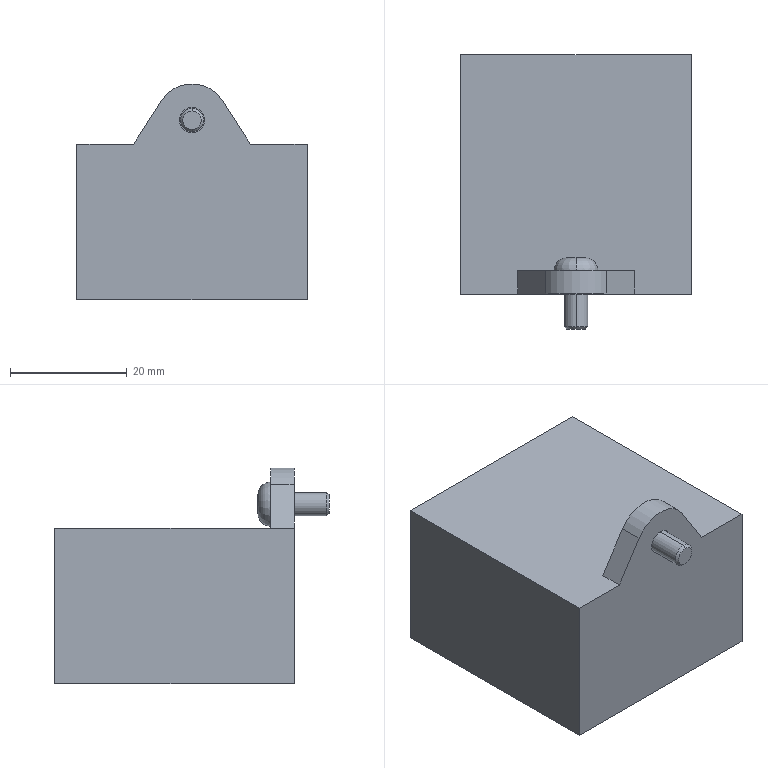Part | SolidWorks | features RefAxis 3, ICE 2, 3DProfileFeature 1, Extrusion 1, RevCut 1, Revolution 1 | 1 solid | 28 faces | box 39.5 x 47 x 37 mm | volume 43916 mm3 | plane 19 | cylinder 5 | torus 2 | cone 2 | commonest cylinder face diameters 4 x2 4.3 x2 12.4 x1
STEP:
#1=CARTESIAN_POINT('',(0.,4.,7.9));
#2=VERTEX_POINT('',#1);
#3=CARTESIAN_POINT('',(0.,4.,0.3));
#4=VERTEX_POINT('',#3);
#5=CARTESIAN_POINT('',(0.,4.,4.1));
#6=DIRECTION('',(0.,1.,0.));
#7=DIRECTION('',(0.,0.,1.));
#8=AXIS2_PLACEMENT_3D('',#5,#6,#7);
#9=CIRCLE('',#8,3.8);
#10=EDGE_CURVE('',#2,#4,#9,.T.);
#11=ORIENTED_EDGE('',*,*,#10,.T.);
#12=CARTESIAN_POINT('',(0.,6.2,2.5));
#13=VERTEX_POINT('',#12);
#14=CARTESIAN_POINT('',(0.,4.,2.5));
#15=DIRECTION('',(1.,0.,0.));
#16=DIRECTION('',(0.,0.,-1.));
#17=AXIS2_PLACEMENT_3D('',#14,#15,#16);
#18=CIRCLE('',#17,2.2);
#19=EDGE_CURVE('',#4,#13,#18,.T.);
#20=ORIENTED_EDGE('',*,*,#19,.T.);
#21=CARTESIAN_POINT('',(0.,6.2,5.7));
#22=VERTEX_POINT('',#21);
#23=CARTESIAN_POINT('',(0.,6.2,4.1));
#24=DIRECTION('',(0.,1.,0.));
#25=DIRECTION('',(0.,0.,1.));
#26=AXIS2_PLACEMENT_3D('',#23,#24,#25);
#27=CIRCLE('',#26,1.6);
#28=EDGE_CURVE('',#22,#13,#27,.T.);
#29=ORIENTED_EDGE('',*,*,#28,.F.);
#30=CARTESIAN_POINT('',(0.,4.,5.7));
#31=DIRECTION('',(-1.,0.,0.));
#32=DIRECTION('',(0.,0.,1.));
#33=AXIS2_PLACEMENT_3D('',#30,#31,#32);
#34=CIRCLE('',#33,2.2);
#35=EDGE_CURVE('',#2,#22,#34,.T.);
#36=ORIENTED_EDGE('',*,*,#35,.F.);
#37=EDGE_LOOP('',(#11,#20,#29,#36));
#38=FACE_OUTER_BOUND('',#37,.T.);
#39=CARTESIAN_POINT('',(0.,4.,4.1));
#40=DIRECTION('',(0.,1.,0.));
#41=DIRECTION('',(0.,0.,1.));
#42=AXIS2_PLACEMENT_3D('',#39,#40,#41);
#43=TOROIDAL_SURFACE('',#42,1.6,2.2);
#44=ADVANCED_FACE('',(#38),#43,.T.);
#45=CARTESIAN_POINT('',(0.,-5.57,6.1));
#46=VERTEX_POINT('',#45);
#47=CARTESIAN_POINT('',(0.,-5.57,2.1));
#48=VERTEX_POINT('',#47);
#49=CARTESIAN_POINT('',(0.,-5.57,4.1));
#50=DIRECTION('',(0.,1.,0.));
#51=DIRECTION('',(0.,0.,1.));
#52=AXIS2_PLACEMENT_3D('',#49,#50,#51);
#53=CIRCLE('',#52,2.);
#54=EDGE_CURVE('',#46,#48,#53,.T.);
#55=ORIENTED_EDGE('',*,*,#54,.T.);
#56=CARTESIAN_POINT('',(0.,4.,2.1));
#57=VERTEX_POINT('',#56);
#58=CARTESIAN_POINT('',(0.,-6.,2.1));
#59=DIRECTION('',(0.,1.,0.));
#60=VECTOR('',#59,1000.);
#61=LINE('',#58,#60);
#62=EDGE_CURVE('',#48,#57,#61,.T.);
#63=ORIENTED_EDGE('',*,*,#62,.T.);
#64=CARTESIAN_POINT('',(0.,4.,6.1));
#65=VERTEX_POINT('',#64);
#66=CARTESIAN_POINT('',(0.,4.,4.1));
#67=DIRECTION('',(0.,1.,0.));
#68=DIRECTION('',(0.,0.,1.));
#69=AXIS2_PLACEMENT_3D('',#66,#67,#68);
#70=CIRCLE('',#69,2.);
#71=EDGE_CURVE('',#65,#57,#70,.T.);
#72=ORIENTED_EDGE('',*,*,#71,.F.);
#73=CARTESIAN_POINT('',(0.,-6.,6.1));
#74=DIRECTION('',(0.,1.,0.));
#75=VECTOR('',#74,1000.);
#76=LINE('',#73,#75);
#77=EDGE_CURVE('',#46,#65,#76,.T.);
#78=ORIENTED_EDGE('',*,*,#77,.F.);
#79=EDGE_LOOP('',(#55,#63,#72,#78));
#80=FACE_OUTER_BOUND('',#79,.T.);
#81=CARTESIAN_POINT('',(0.,-6.,4.1));
#82=DIRECTION('',(0.,1.,0.));
#83=DIRECTION('',(0.,0.,1.));
#84=AXIS2_PLACEMENT_3D('',#81,#82,#83);
#85=CYLINDRICAL_SURFACE('',#84,2.);
#86=ADVANCED_FACE('',(#80),#85,.T.);
#87=CARTESIAN_POINT('',(0.,-6.,5.671));
#88=VERTEX_POINT('',#87);
#89=CARTESIAN_POINT('',(0.,-6.,2.53));
#90=VERTEX_POINT('',#89);
#91=CARTESIAN_POINT('',(0.,-6.,4.1));
#92=DIRECTION('',(0.,1.,0.));
#93=DIRECTION('',(0.,0.,1.));
#94=AXIS2_PLACEMENT_3D('',#91,#92,#93);
#95=CIRCLE('',#94,1.57);
#96=EDGE_CURVE('',#88,#90,#95,.T.);
#97=ORIENTED_EDGE('',*,*,#96,.T.);
#98=CARTESIAN_POINT('',(0.,-6.,2.53));
#99=DIRECTION('',(0.,0.7071,-0.7071));
#100=VECTOR('',#99,1000.);
#101=LINE('',#98,#100);
#102=EDGE_CURVE('',#90,#48,#101,.T.);
#103=ORIENTED_EDGE('',*,*,#102,.T.);
#104=ORIENTED_EDGE('',*,*,#54,.F.);
#105=CARTESIAN_POINT('',(0.,-6.,5.671));
#106=DIRECTION('',(0.,0.7071,0.7071));
#107=VECTOR('',#106,1000.);
#108=LINE('',#105,#107);
#109=EDGE_CURVE('',#88,#46,#108,.T.);
#110=ORIENTED_EDGE('',*,*,#109,.F.);
#111=EDGE_LOOP('',(#97,#103,#104,#110));
#112=FACE_OUTER_BOUND('',#111,.T.);
#113=CARTESIAN_POINT('',(0.,-6.,4.1));
#114=DIRECTION('',(0.,1.,0.));
#115=DIRECTION('',(0.,0.,1.));
#116=AXIS2_PLACEMENT_3D('',#113,#114,#115);
#117=CONICAL_SURFACE('',#116,1.57,0.7854);
#118=ADVANCED_FACE('',(#112),#117,.T.);
#119=CARTESIAN_POINT('',(0.,0.,1.95));
#120=VERTEX_POINT('',#119);
#121=CARTESIAN_POINT('',(0.,0.,6.25));
#122=VERTEX_POINT('',#121);
#123=CARTESIAN_POINT('',(0.,0.,4.1));
#124=DIRECTION('',(0.,1.,0.));
#125=DIRECTION('',(0.,0.,1.));
#126=AXIS2_PLACEMENT_3D('',#123,#124,#125);
#127=CIRCLE('',#126,2.15);
#128=EDGE_CURVE('',#120,#122,#127,.T.);
#129=ORIENTED_EDGE('',*,*,#128,.F.);
#130=CARTESIAN_POINT('',(0.,4.,1.95));
#131=VERTEX_POINT('',#130);
#132=CARTESIAN_POINT('',(0.,0.,1.95));
#133=DIRECTION('',(0.,1.,0.));
#134=VECTOR('',#133,1000.);
#135=LINE('',#132,#134);
#136=EDGE_CURVE('',#120,#131,#135,.T.);
#137=ORIENTED_EDGE('',*,*,#136,.T.);
#138=CARTESIAN_POINT('',(0.,4.,6.25));
#139=VERTEX_POINT('',#138);
#140=CARTESIAN_POINT('',(0.,4.,4.1));
#141=DIRECTION('',(0.,1.,0.));
#142=DIRECTION('',(0.,0.,1.));
#143=AXIS2_PLACEMENT_3D('',#140,#141,#142);
#144=CIRCLE('',#143,2.15);
#145=EDGE_CURVE('',#131,#139,#144,.T.);
#146=ORIENTED_EDGE('',*,*,#145,.T.);
#147=CARTESIAN_POINT('',(0.,0.,6.25));
#148=DIRECTION('',(0.,1.,0.));
#149=VECTOR('',#148,1000.);
#150=LINE('',#147,#149);
#151=EDGE_CURVE('',#122,#139,#150,.T.);
#152=ORIENTED_EDGE('',*,*,#151,.F.);
#153=EDGE_LOOP('',(#129,#137,#146,#152));
#154=FACE_OUTER_BOUND('',#153,.T.);
#155=CARTESIAN_POINT('',(0.,0.,4.1));
#156=DIRECTION('',(0.,1.,0.));
#157=DIRECTION('',(0.,0.,1.));
#158=AXIS2_PLACEMENT_3D('',#155,#156,#157);
#159=CYLINDRICAL_SURFACE('',#158,2.15);
#160=ADVANCED_FACE('',(#154),#159,.F.);
#161=CARTESIAN_POINT('',(10.,4.,0.));
#162=VERTEX_POINT('',#161);
#163=CARTESIAN_POINT('',(-10.,4.,0.));
#164=VERTEX_POINT('',#163);
#165=CARTESIAN_POINT('',(10.,4.,0.));
#166=DIRECTION('',(-1.,0.,0.));
#167=VECTOR('',#166,1000.);
#168=LINE('',#165,#167);
#169=EDGE_CURVE('',#162,#164,#168,.T.);
#170=ORIENTED_EDGE('',*,*,#169,.T.);
#171=CARTESIAN_POINT('',(-5.217,4.,7.45));
#172=VERTEX_POINT('',#171);
#173=CARTESIAN_POINT('',(-10.,4.,0.));
#174=DIRECTION('',(0.5403,0.,0.8415));
#175=VECTOR('',#174,1000.);
#176=LINE('',#173,#175);
#177=EDGE_CURVE('',#164,#172,#176,.T.);
#178=ORIENTED_EDGE('',*,*,#177,.T.);
#179=CARTESIAN_POINT('',(5.217,4.,7.45));
#180=VERTEX_POINT('',#179);
#181=CARTESIAN_POINT('',(0.,4.,4.1));
#182=DIRECTION('',(0.,1.,0.));
#183=DIRECTION('',(0.,0.,1.));
#184=AXIS2_PLACEMENT_3D('',#181,#182,#183);
#185=CIRCLE('',#184,6.2);
#186=EDGE_CURVE('',#172,#180,#185,.T.);
#187=ORIENTED_EDGE('',*,*,#186,.T.);
#188=CARTESIAN_POINT('',(5.217,4.,7.45));
#189=DIRECTION('',(0.5403,0.,-0.8415));
#190=VECTOR('',#189,1000.);
#191=LINE('',#188,#190);
#192=EDGE_CURVE('',#180,#162,#191,.T.);
#193=ORIENTED_EDGE('',*,*,#192,.T.);
#194=EDGE_LOOP('',(#170,#178,#187,#193));
#195=FACE_OUTER_BOUND('',#194,.T.);
#196=ORIENTED_EDGE('',*,*,#10,.F.);
#197=CARTESIAN_POINT('',(0.,4.,4.1));
#198=DIRECTION('',(0.,1.,0.));
#199=DIRECTION('',(0.,0.,1.));
#200=AXIS2_PLACEMENT_3D('',#197,#198,#199);
#201=CIRCLE('',#200,3.8);
#202=EDGE_CURVE('',#4,#2,#201,.T.);
#203=ORIENTED_EDGE('',*,*,#202,.F.);
#204=EDGE_LOOP('',(#196,#203));
#205=FACE_BOUND('',#204,.T.);
#206=CARTESIAN_POINT('',(0.,4.,4.1));
#207=DIRECTION('',(0.,1.,0.));
#208=DIRECTION('',(0.,0.,1.));
#209=AXIS2_PLACEMENT_3D('',#206,#207,#208);
#210=PLANE('',#209);
#211=ADVANCED_FACE('',(#195,#205),#210,.T.);
#212=CARTESIAN_POINT('',(-19.75,0.,-26.7));
#213=VERTEX_POINT('',#212);
#214=CARTESIAN_POINT('',(-19.75,0.,0.));
#215=VERTEX_POINT('',#214);
#216=CARTESIAN_POINT('',(-19.75,0.,-26.7));
#217=DIRECTION('',(0.,0.,1.));
#218=VECTOR('',#217,1000.);
#219=LINE('',#216,#218);
#220=EDGE_CURVE('',#213,#215,#219,.T.);
#221=ORIENTED_EDGE('',*,*,#220,.F.);
#222=CARTESIAN_POINT('',(19.75,0.,-26.7));
#223=VERTEX_POINT('',#222);
#224=CARTESIAN_POINT('',(19.75,0.,-26.7));
#225=DIRECTION('',(-1.,0.,0.));
#226=VECTOR('',#225,1000.);
#227=LINE('',#224,#226);
#228=EDGE_CURVE('',#223,#213,#227,.T.);
#229=ORIENTED_EDGE('',*,*,#228,.F.);
#230=CARTESIAN_POINT('',(19.75,0.,0.));
#231=VERTEX_POINT('',#230);
#232=CARTESIAN_POINT('',(19.75,0.,0.));
#233=DIRECTION('',(0.,0.,-1.));
#234=VECTOR('',#233,1000.);
#235=LINE('',#232,#234);
#236=EDGE_CURVE('',#231,#223,#235,.T.);
#237=ORIENTED_EDGE('',*,*,#236,.F.);
#238=CARTESIAN_POINT('',(10.,0.,0.));
#239=VERTEX_POINT('',#238);
#240=CARTESIAN_POINT('',(-19.75,0.,0.));
#241=DIRECTION('',(1.,0.,0.));
#242=VECTOR('',#241,1000.);
#243=LINE('',#240,#242);
#244=EDGE_CURVE('',#239,#231,#243,.T.);
#245=ORIENTED_EDGE('',*,*,#244,.F.);
#246=CARTESIAN_POINT('',(5.217,0.,7.45));
#247=VERTEX_POINT('',#246);
#248=CARTESIAN_POINT('',(5.217,0.,7.45));
#249=DIRECTION('',(0.5403,0.,-0.8415));
#250=VECTOR('',#249,1000.);
#251=LINE('',#248,#250);
#252=EDGE_CURVE('',#247,#239,#251,.T.);
#253=ORIENTED_EDGE('',*,*,#252,.F.);
#254=CARTESIAN_POINT('',(-5.217,0.,7.45));
#255=VERTEX_POINT('',#254);
#256=CARTESIAN_POINT('',(0.,0.,4.1));
#257=DIRECTION('',(0.,1.,0.));
#258=DIRECTION('',(0.,0.,1.));
#259=AXIS2_PLACEMENT_3D('',#256,#257,#258);
#260=CIRCLE('',#259,6.2);
#261=EDGE_CURVE('',#255,#247,#260,.T.);
#262=ORIENTED_EDGE('',*,*,#261,.F.);
#263=CARTESIAN_POINT('',(-10.,0.,0.));
#264=VERTEX_POINT('',#263);
#265=CARTESIAN_POINT('',(-10.,0.,0.));
#266=DIRECTION('',(0.5403,0.,0.8415));
#267=VECTOR('',#266,1000.);
#268=LINE('',#265,#267);
#269=EDGE_CURVE('',#264,#255,#268,.T.);
#270=ORIENTED_EDGE('',*,*,#269,.F.);
#271=CARTESIAN_POINT('',(-19.75,0.,0.));
#272=DIRECTION('',(1.,0.,0.));
#273=VECTOR('',#272,1000.);
#274=LINE('',#271,#273);
#275=EDGE_CURVE('',#215,#264,#274,.T.);
#276=ORIENTED_EDGE('',*,*,#275,.F.);
#277=EDGE_LOOP('',(#221,#229,#237,#245,#253,#262,#270,#276));
#278=FACE_OUTER_BOUND('',#277,.T.);
#279=CARTESIAN_POINT('',(0.,0.,4.1));
#280=DIRECTION('',(0.,1.,0.));
#281=DIRECTION('',(0.,0.,1.));
#282=AXIS2_PLACEMENT_3D('',#279,#280,#281);
#283=CIRCLE('',#282,2.15);
#284=EDGE_CURVE('',#122,#120,#283,.T.);
#285=ORIENTED_EDGE('',*,*,#284,.T.);
#286=ORIENTED_EDGE('',*,*,#128,.T.);
#287=EDGE_LOOP('',(#285,#286));
#288=FACE_BOUND('',#287,.T.);
#289=CARTESIAN_POINT('',(0.,0.,0.));
#290=DIRECTION('',(0.,1.,0.));
#291=DIRECTION('',(0.,0.,1.));
#292=AXIS2_PLACEMENT_3D('',#289,#290,#291);
#293=PLANE('',#292);
#294=ADVANCED_FACE('',(#278,#288),#293,.F.);
#295=CARTESIAN_POINT('',(-10.,4.,0.));
#296=DIRECTION('',(0.,-1.,0.));
#297=VECTOR('',#296,1000.);
#298=LINE('',#295,#297);
#299=EDGE_CURVE('',#164,#264,#298,.T.);
#300=ORIENTED_EDGE('',*,*,#299,.F.);
#301=ORIENTED_EDGE('',*,*,#169,.F.);
#302=CARTESIAN_POINT('',(10.,4.,0.));
#303=DIRECTION('',(0.,-1.,0.));
#304=VECTOR('',#303,1000.);
#305=LINE('',#302,#304);
#306=EDGE_CURVE('',#162,#239,#305,.T.);
#307=ORIENTED_EDGE('',*,*,#306,.T.);
#308=ORIENTED_EDGE('',*,*,#244,.T.);
#309=CARTESIAN_POINT('',(19.75,41.,0.));
#310=VERTEX_POINT('',#309);
#311=CARTESIAN_POINT('',(19.75,41.,0.));
#312=DIRECTION('',(0.,-1.,0.));
#313=VECTOR('',#312,1000.);
#314=LINE('',#311,#313);
#315=EDGE_CURVE('',#310,#231,#314,.T.);
#316=ORIENTED_EDGE('',*,*,#315,.F.);
#317=CARTESIAN_POINT('',(-19.75,41.,0.));
#318=VERTEX_POINT('',#317);
#319=CARTESIAN_POINT('',(-19.75,41.,0.));
#320=DIRECTION('',(1.,0.,0.));
#321=VECTOR('',#320,1000.);
#322=LINE('',#319,#321);
#323=EDGE_CURVE('',#318,#310,#322,.T.);
#324=ORIENTED_EDGE('',*,*,#323,.F.);
#325=CARTESIAN_POINT('',(-19.75,41.,0.));
#326=DIRECTION('',(0.,-1.,0.));
#327=VECTOR('',#326,1000.);
#328=LINE('',#325,#327);
#329=EDGE_CURVE('',#318,#215,#328,.T.);
#330=ORIENTED_EDGE('',*,*,#329,.T.);
#331=ORIENTED_EDGE('',*,*,#275,.T.);
#332=EDGE_LOOP('',(#300,#301,#307,#308,#316,#324,#330,#331));
#333=FACE_OUTER_BOUND('',#332,.T.);
#334=CARTESIAN_POINT('',(-19.75,41.,0.));
#335=DIRECTION('',(0.,0.,-1.));
#336=DIRECTION('',(-1.,0.,0.));
#337=AXIS2_PLACEMENT_3D('',#334,#335,#336);
#338=PLANE('',#337);
#339=ADVANCED_FACE('',(#333),#338,.F.);
#340=ORIENTED_EDGE('',*,*,#220,.T.);
#341=ORIENTED_EDGE('',*,*,#329,.F.);
#342=CARTESIAN_POINT('',(-19.75,41.,-26.7));
#343=VERTEX_POINT('',#342);
#344=CARTESIAN_POINT('',(-19.75,41.,-26.7));
#345=DIRECTION('',(0.,0.,1.));
#346=VECTOR('',#345,1000.);
#347=LINE('',#344,#346);
#348=EDGE_CURVE('',#343,#318,#347,.T.);
#349=ORIENTED_EDGE('',*,*,#348,.F.);
#350=CARTESIAN_POINT('',(-19.75,41.,-26.7));
#351=DIRECTION('',(0.,-1.,0.));
#352=VECTOR('',#351,1000.);
#353=LINE('',#350,#352);
#354=EDGE_CURVE('',#343,#213,#353,.T.);
#355=ORIENTED_EDGE('',*,*,#354,.T.);
#356=EDGE_LOOP('',(#340,#341,#349,#355));
#357=FACE_OUTER_BOUND('',#356,.T.);
#358=CARTESIAN_POINT('',(-19.75,41.,-26.7));
#359=DIRECTION('',(1.,0.,0.));
#360=DIRECTION('',(0.,0.,-1.));
#361=AXIS2_PLACEMENT_3D('',#358,#359,#360);
#362=PLANE('',#361);
#363=ADVANCED_FACE('',(#357),#362,.F.);
#364=ORIENTED_EDGE('',*,*,#236,.T.);
#365=CARTESIAN_POINT('',(19.75,41.,-26.7));
#366=VERTEX_POINT('',#365);
#367=CARTESIAN_POINT('',(19.75,41.,-26.7));
#368=DIRECTION('',(0.,-1.,0.));
#369=VECTOR('',#368,1000.);
#370=LINE('',#367,#369);
#371=EDGE_CURVE('',#366,#223,#370,.T.);
#372=ORIENTED_EDGE('',*,*,#371,.F.);
#373=CARTESIAN_POINT('',(19.75,41.,0.));
#374=DIRECTION('',(0.,0.,-1.));
#375=VECTOR('',#374,1000.);
#376=LINE('',#373,#375);
#377=EDGE_CURVE('',#310,#366,#376,.T.);
#378=ORIENTED_EDGE('',*,*,#377,.F.);
#379=ORIENTED_EDGE('',*,*,#315,.T.);
#380=EDGE_LOOP('',(#364,#372,#378,#379));
#381=FACE_OUTER_BOUND('',#380,.T.);
#382=CARTESIAN_POINT('',(19.75,41.,0.));
#383=DIRECTION('',(-1.,0.,0.));
#384=DIRECTION('',(0.,0.,1.));
#385=AXIS2_PLACEMENT_3D('',#382,#383,#384);
#386=PLANE('',#385);
#387=ADVANCED_FACE('',(#381),#386,.F.);
#388=ORIENTED_EDGE('',*,*,#228,.T.);
#389=ORIENTED_EDGE('',*,*,#354,.F.);
#390=CARTESIAN_POINT('',(19.75,41.,-26.7));
#391=DIRECTION('',(-1.,0.,0.));
#392=VECTOR('',#391,1000.);
#393=LINE('',#390,#392);
#394=EDGE_CURVE('',#366,#343,#393,.T.);
#395=ORIENTED_EDGE('',*,*,#394,.F.);
#396=ORIENTED_EDGE('',*,*,#371,.T.);
#397=EDGE_LOOP('',(#388,#389,#395,#396));
#398=FACE_OUTER_BOUND('',#397,.T.);
#399=CARTESIAN_POINT('',(19.75,41.,-26.7));
#400=DIRECTION('',(0.,0.,1.));
#401=DIRECTION('',(1.,0.,0.));
#402=AXIS2_PLACEMENT_3D('',#399,#400,#401);
#403=PLANE('',#402);
#404=ADVANCED_FACE('',(#398),#403,.F.);
#405=ORIENTED_EDGE('',*,*,#348,.T.);
#406=ORIENTED_EDGE('',*,*,#323,.T.);
#407=ORIENTED_EDGE('',*,*,#377,.T.);
#408=ORIENTED_EDGE('',*,*,#394,.T.);
#409=EDGE_LOOP('',(#405,#406,#407,#408));
#410=FACE_OUTER_BOUND('',#409,.T.);
#411=CARTESIAN_POINT('',(0.,41.,0.));
#412=DIRECTION('',(0.,1.,0.));
#413=DIRECTION('',(0.,0.,1.));
#414=AXIS2_PLACEMENT_3D('',#411,#412,#413);
#415=PLANE('',#414);
#416=ADVANCED_FACE('',(#410),#415,.T.);
#417=ORIENTED_EDGE('',*,*,#269,.T.);
#418=CARTESIAN_POINT('',(-5.217,4.,7.45));
#419=DIRECTION('',(0.,-1.,0.));
#420=VECTOR('',#419,1000.);
#421=LINE('',#418,#420);
#422=EDGE_CURVE('',#172,#255,#421,.T.);
#423=ORIENTED_EDGE('',*,*,#422,.F.);
#424=ORIENTED_EDGE('',*,*,#177,.F.);
#425=ORIENTED_EDGE('',*,*,#299,.T.);
#426=EDGE_LOOP('',(#417,#423,#424,#425));
#427=FACE_OUTER_BOUND('',#426,.T.);
#428=CARTESIAN_POINT('',(-10.,4.,0.));
#429=DIRECTION('',(0.8415,0.,-0.5403));
#430=DIRECTION('',(-0.5403,0.,-0.8415));
#431=AXIS2_PLACEMENT_3D('',#428,#429,#430);
#432=PLANE('',#431);
#433=ADVANCED_FACE('',(#427),#432,.F.);
#434=ORIENTED_EDGE('',*,*,#261,.T.);
#435=CARTESIAN_POINT('',(5.217,4.,7.45));
#436=DIRECTION('',(0.,-1.,0.));
#437=VECTOR('',#436,1000.);
#438=LINE('',#435,#437);
#439=EDGE_CURVE('',#180,#247,#438,.T.);
#440=ORIENTED_EDGE('',*,*,#439,.F.);
#441=ORIENTED_EDGE('',*,*,#186,.F.);
#442=ORIENTED_EDGE('',*,*,#422,.T.);
#443=EDGE_LOOP('',(#434,#440,#441,#442));
#444=FACE_OUTER_BOUND('',#443,.T.);
#445=CARTESIAN_POINT('',(0.,4.,4.1));
#446=DIRECTION('',(0.,-1.,0.));
#447=DIRECTION('',(0.,0.,-1.));
#448=AXIS2_PLACEMENT_3D('',#445,#446,#447);
#449=CYLINDRICAL_SURFACE('',#448,6.2);
#450=ADVANCED_FACE('',(#444),#449,.T.);
#451=ORIENTED_EDGE('',*,*,#252,.T.);
#452=ORIENTED_EDGE('',*,*,#306,.F.);
#453=ORIENTED_EDGE('',*,*,#192,.F.);
#454=ORIENTED_EDGE('',*,*,#439,.T.);
#455=EDGE_LOOP('',(#451,#452,#453,#454));
#456=FACE_OUTER_BOUND('',#455,.T.);
#457=CARTESIAN_POINT('',(5.217,4.,7.45));
#458=DIRECTION('',(-0.8415,0.,-0.5403));
#459=DIRECTION('',(-0.5403,0.,0.8415));
#460=AXIS2_PLACEMENT_3D('',#457,#458,#459);
#461=PLANE('',#460);
#462=ADVANCED_FACE('',(#456),#461,.F.);
#463=ORIENTED_EDGE('',*,*,#136,.F.);
#464=ORIENTED_EDGE('',*,*,#284,.F.);
#465=ORIENTED_EDGE('',*,*,#151,.T.);
#466=CARTESIAN_POINT('',(0.,4.,4.1));
#467=DIRECTION('',(0.,1.,0.));
#468=DIRECTION('',(0.,0.,1.));
#469=AXIS2_PLACEMENT_3D('',#466,#467,#468);
#470=CIRCLE('',#469,2.15);
#471=EDGE_CURVE('',#139,#131,#470,.T.);
#472=ORIENTED_EDGE('',*,*,#471,.T.);
#473=EDGE_LOOP('',(#463,#464,#465,#472));
#474=FACE_OUTER_BOUND('',#473,.T.);
#475=CARTESIAN_POINT('',(0.,0.,4.1));
#476=DIRECTION('',(0.,1.,0.));
#477=DIRECTION('',(0.,0.,1.));
#478=AXIS2_PLACEMENT_3D('',#475,#476,#477);
#479=CYLINDRICAL_SURFACE('',#478,2.15);
#480=ADVANCED_FACE('',(#474),#479,.F.);
#481=ORIENTED_EDGE('',*,*,#96,.F.);
#482=CARTESIAN_POINT('',(0.,-6.,4.1));
#483=DIRECTION('',(0.,1.,0.));
#484=DIRECTION('',(0.,0.,1.));
#485=AXIS2_PLACEMENT_3D('',#482,#483,#484);
#486=CIRCLE('',#485,1.57);
#487=EDGE_CURVE('',#90,#88,#486,.T.);
#488=ORIENTED_EDGE('',*,*,#487,.F.);
#489=EDGE_LOOP('',(#481,#488));
#490=FACE_OUTER_BOUND('',#489,.T.);
#491=CARTESIAN_POINT('',(1.571,-6.,4.1));
#492=DIRECTION('',(0.,1.,0.));
#493=DIRECTION('',(0.,0.,1.));
#494=AXIS2_PLACEMENT_3D('',#491,#492,#493);
#495=PLANE('',#494);
#496=ADVANCED_FACE('',(#490),#495,.F.);
#497=ORIENTED_EDGE('',*,*,#102,.F.);
#498=ORIENTED_EDGE('',*,*,#487,.T.);
#499=ORIENTED_EDGE('',*,*,#109,.T.);
#500=CARTESIAN_POINT('',(0.,-5.57,4.1));
#501=DIRECTION('',(0.,1.,0.));
#502=DIRECTION('',(0.,0.,1.));
#503=AXIS2_PLACEMENT_3D('',#500,#501,#502);
#504=CIRCLE('',#503,2.);
#505=EDGE_CURVE('',#48,#46,#504,.T.);
#506=ORIENTED_EDGE('',*,*,#505,.F.);
#507=EDGE_LOOP('',(#497,#498,#499,#506));
#508=FACE_OUTER_BOUND('',#507,.T.);
#509=CARTESIAN_POINT('',(0.,-6.,4.1));
#510=DIRECTION('',(0.,1.,0.));
#511=DIRECTION('',(0.,0.,1.));
#512=AXIS2_PLACEMENT_3D('',#509,#510,#511);
#513=CONICAL_SURFACE('',#512,1.57,0.7854);
#514=ADVANCED_FACE('',(#508),#513,.T.);
#515=ORIENTED_EDGE('',*,*,#62,.F.);
#516=ORIENTED_EDGE('',*,*,#505,.T.);
#517=ORIENTED_EDGE('',*,*,#77,.T.);
#518=CARTESIAN_POINT('',(0.,4.,4.1));
#519=DIRECTION('',(0.,1.,0.));
#520=DIRECTION('',(0.,0.,1.));
#521=AXIS2_PLACEMENT_3D('',#518,#519,#520);
#522=CIRCLE('',#521,2.);
#523=EDGE_CURVE('',#57,#65,#522,.T.);
#524=ORIENTED_EDGE('',*,*,#523,.F.);
#525=EDGE_LOOP('',(#515,#516,#517,#524));
#526=FACE_OUTER_BOUND('',#525,.T.);
#527=CARTESIAN_POINT('',(0.,-6.,4.1));
#528=DIRECTION('',(0.,1.,0.));
#529=DIRECTION('',(0.,0.,1.));
#530=AXIS2_PLACEMENT_3D('',#527,#528,#529);
#531=CYLINDRICAL_SURFACE('',#530,2.);
#532=ADVANCED_FACE('',(#526),#531,.T.);
#533=ORIENTED_EDGE('',*,*,#471,.F.);
#534=ORIENTED_EDGE('',*,*,#145,.F.);
#535=EDGE_LOOP('',(#533,#534));
#536=FACE_OUTER_BOUND('',#535,.T.);
#537=ORIENTED_EDGE('',*,*,#71,.T.);
#538=ORIENTED_EDGE('',*,*,#523,.T.);
#539=EDGE_LOOP('',(#537,#538));
#540=FACE_BOUND('',#539,.T.);
#541=CARTESIAN_POINT('',(3.8,4.,4.1));
#542=DIRECTION('',(0.,1.,0.));
#543=DIRECTION('',(0.,0.,1.));
#544=AXIS2_PLACEMENT_3D('',#541,#542,#543);
#545=PLANE('',#544);
#546=ADVANCED_FACE('',(#536,#540),#545,.F.);
#547=CARTESIAN_POINT('',(-1.25,6.2,3.378));
#548=VERTEX_POINT('',#547);
#549=CARTESIAN_POINT('',(-1.25,6.2,4.822));
#550=VERTEX_POINT('',#549);
#551=CARTESIAN_POINT('',(-1.25,6.2,3.378));
#552=DIRECTION('',(0.,0.,1.));
#553=VECTOR('',#552,1000.);
#554=LINE('',#551,#553);
#555=EDGE_CURVE('',#548,#550,#554,.T.);
#556=ORIENTED_EDGE('',*,*,#555,.F.);
#557=CARTESIAN_POINT('',(0.,6.2,2.657));
#558=VERTEX_POINT('',#557);
#559=CARTESIAN_POINT('',(0.,6.2,2.657));
#560=DIRECTION('',(-0.866,0.,0.5));
#561=VECTOR('',#560,1000.);
#562=LINE('',#559,#561);
#563=EDGE_CURVE('',#558,#548,#562,.T.);
#564=ORIENTED_EDGE('',*,*,#563,.F.);
#565=CARTESIAN_POINT('',(1.25,6.2,3.378));
#566=VERTEX_POINT('',#565);
#567=CARTESIAN_POINT('',(1.25,6.2,3.378));
#568=DIRECTION('',(-0.866,0.,-0.5));
#569=VECTOR('',#568,1000.);
#570=LINE('',#567,#569);
#571=EDGE_CURVE('',#566,#558,#570,.T.);
#572=ORIENTED_EDGE('',*,*,#571,.F.);
#573=CARTESIAN_POINT('',(1.25,6.2,4.822));
#574=VERTEX_POINT('',#573);
#575=CARTESIAN_POINT('',(1.25,6.2,4.822));
#576=DIRECTION('',(0.,0.,-1.));
#577=VECTOR('',#576,1000.);
#578=LINE('',#575,#577);
#579=EDGE_CURVE('',#574,#566,#578,.T.);
#580=ORIENTED_EDGE('',*,*,#579,.F.);
#581=CARTESIAN_POINT('',(0.,6.2,5.543));
#582=VERTEX_POINT('',#581);
#583=CARTESIAN_POINT('',(0.,6.2,5.543));
#584=DIRECTION('',(0.866,0.,-0.5));
#585=VECTOR('',#584,1000.);
#586=LINE('',#583,#585);
#587=EDGE_CURVE('',#582,#574,#586,.T.);
#588=ORIENTED_EDGE('',*,*,#587,.F.);
#589=CARTESIAN_POINT('',(-1.25,6.2,4.822));
#590=DIRECTION('',(0.866,0.,0.5));
#591=VECTOR('',#590,1000.);
#592=LINE('',#589,#591);
#593=EDGE_CURVE('',#550,#582,#592,.T.);
#594=ORIENTED_EDGE('',*,*,#593,.F.);
#595=EDGE_LOOP('',(#556,#564,#572,#580,#588,#594));
#596=FACE_BOUND('',#595,.T.);
#597=ORIENTED_EDGE('',*,*,#28,.T.);
#598=CARTESIAN_POINT('',(0.,6.2,4.1));
#599=DIRECTION('',(0.,1.,0.));
#600=DIRECTION('',(0.,0.,1.));
#601=AXIS2_PLACEMENT_3D('',#598,#599,#600);
#602=CIRCLE('',#601,1.6);
#603=EDGE_CURVE('',#13,#22,#602,.T.);
#604=ORIENTED_EDGE('',*,*,#603,.T.);
#605=EDGE_LOOP('',(#597,#604));
#606=FACE_OUTER_BOUND('',#605,.T.);
#607=CARTESIAN_POINT('',(0.,6.2,4.1));
#608=DIRECTION('',(0.,-1.,0.));
#609=DIRECTION('',(0.,0.,-1.));
#610=AXIS2_PLACEMENT_3D('',#607,#608,#609);
#611=PLANE('',#610);
#612=ADVANCED_FACE('',(#596,#606),#611,.F.);
#613=ORIENTED_EDGE('',*,*,#19,.F.);
#614=ORIENTED_EDGE('',*,*,#202,.T.);
#615=ORIENTED_EDGE('',*,*,#35,.T.);
#616=ORIENTED_EDGE('',*,*,#603,.F.);
#617=EDGE_LOOP('',(#613,#614,#615,#616));
#618=FACE_OUTER_BOUND('',#617,.T.);
#619=CARTESIAN_POINT('',(0.,4.,4.1));
#620=DIRECTION('',(0.,1.,0.));
#621=DIRECTION('',(0.,0.,1.));
#622=AXIS2_PLACEMENT_3D('',#619,#620,#621);
#623=TOROIDAL_SURFACE('',#622,1.6,2.2);
#624=ADVANCED_FACE('',(#618),#623,.T.);
#625=ORIENTED_EDGE('',*,*,#563,.T.);
#626=CARTESIAN_POINT('',(-1.25,4.9,3.378));
#627=VERTEX_POINT('',#626);
#628=CARTESIAN_POINT('',(-1.25,4.9,3.378));
#629=DIRECTION('',(0.,1.,0.));
#630=VECTOR('',#629,1000.);
#631=LINE('',#628,#630);
#632=EDGE_CURVE('',#627,#548,#631,.T.);
#633=ORIENTED_EDGE('',*,*,#632,.F.);
#634=CARTESIAN_POINT('',(0.,4.9,2.657));
#635=VERTEX_POINT('',#634);
#636=CARTESIAN_POINT('',(0.,4.9,2.657));
#637=DIRECTION('',(-0.866,0.,0.5));
#638=VECTOR('',#637,1000.);
#639=LINE('',#636,#638);
#640=EDGE_CURVE('',#635,#627,#639,.T.);
#641=ORIENTED_EDGE('',*,*,#640,.F.);
#642=CARTESIAN_POINT('',(0.,4.9,2.657));
#643=DIRECTION('',(0.,1.,0.));
#644=VECTOR('',#643,1000.);
#645=LINE('',#642,#644);
#646=EDGE_CURVE('',#635,#558,#645,.T.);
#647=ORIENTED_EDGE('',*,*,#646,.T.);
#648=EDGE_LOOP('',(#625,#633,#641,#647));
#649=FACE_OUTER_BOUND('',#648,.T.);
#650=CARTESIAN_POINT('',(0.,4.9,2.657));
#651=DIRECTION('',(-0.5,0.,-0.866));
#652=DIRECTION('',(-0.866,0.,0.5));
#653=AXIS2_PLACEMENT_3D('',#650,#651,#652);
#654=PLANE('',#653);
#655=ADVANCED_FACE('',(#649),#654,.F.);
#656=ORIENTED_EDGE('',*,*,#571,.T.);
#657=ORIENTED_EDGE('',*,*,#646,.F.);
#658=CARTESIAN_POINT('',(1.25,4.9,3.378));
#659=VERTEX_POINT('',#658);
#660=CARTESIAN_POINT('',(1.25,4.9,3.378));
#661=DIRECTION('',(-0.866,0.,-0.5));
#662=VECTOR('',#661,1000.);
#663=LINE('',#660,#662);
#664=EDGE_CURVE('',#659,#635,#663,.T.);
#665=ORIENTED_EDGE('',*,*,#664,.F.);
#666=CARTESIAN_POINT('',(1.25,4.9,3.378));
#667=DIRECTION('',(0.,1.,0.));
#668=VECTOR('',#667,1000.);
#669=LINE('',#666,#668);
#670=EDGE_CURVE('',#659,#566,#669,.T.);
#671=ORIENTED_EDGE('',*,*,#670,.T.);
#672=EDGE_LOOP('',(#656,#657,#665,#671));
#673=FACE_OUTER_BOUND('',#672,.T.);
#674=CARTESIAN_POINT('',(1.25,4.9,3.378));
#675=DIRECTION('',(0.5,0.,-0.866));
#676=DIRECTION('',(-0.866,0.,-0.5));
#677=AXIS2_PLACEMENT_3D('',#674,#675,#676);
#678=PLANE('',#677);
#679=ADVANCED_FACE('',(#673),#678,.F.);
#680=ORIENTED_EDGE('',*,*,#579,.T.);
#681=ORIENTED_EDGE('',*,*,#670,.F.);
#682=CARTESIAN_POINT('',(1.25,4.9,4.822));
#683=VERTEX_POINT('',#682);
#684=CARTESIAN_POINT('',(1.25,4.9,4.822));
#685=DIRECTION('',(0.,0.,-1.));
#686=VECTOR('',#685,1000.);
#687=LINE('',#684,#686);
#688=EDGE_CURVE('',#683,#659,#687,.T.);
#689=ORIENTED_EDGE('',*,*,#688,.F.);
#690=CARTESIAN_POINT('',(1.25,4.9,4.822));
#691=DIRECTION('',(0.,1.,0.));
#692=VECTOR('',#691,1000.);
#693=LINE('',#690,#692);
#694=EDGE_CURVE('',#683,#574,#693,.T.);
#695=ORIENTED_EDGE('',*,*,#694,.T.);
#696=EDGE_LOOP('',(#680,#681,#689,#695));
#697=FACE_OUTER_BOUND('',#696,.T.);
#698=CARTESIAN_POINT('',(1.25,4.9,4.822));
#699=DIRECTION('',(1.,0.,0.));
#700=DIRECTION('',(0.,0.,-1.));
#701=AXIS2_PLACEMENT_3D('',#698,#699,#700);
#702=PLANE('',#701);
#703=ADVANCED_FACE('',(#697),#702,.F.);
#704=ORIENTED_EDGE('',*,*,#587,.T.);
#705=ORIENTED_EDGE('',*,*,#694,.F.);
#706=CARTESIAN_POINT('',(0.,4.9,5.543));
#707=VERTEX_POINT('',#706);
#708=CARTESIAN_POINT('',(0.,4.9,5.543));
#709=DIRECTION('',(0.866,0.,-0.5));
#710=VECTOR('',#709,1000.);
#711=LINE('',#708,#710);
#712=EDGE_CURVE('',#707,#683,#711,.T.);
#713=ORIENTED_EDGE('',*,*,#712,.F.);
#714=CARTESIAN_POINT('',(0.,4.9,5.543));
#715=DIRECTION('',(0.,1.,0.));
#716=VECTOR('',#715,1000.);
#717=LINE('',#714,#716);
#718=EDGE_CURVE('',#707,#582,#717,.T.);
#719=ORIENTED_EDGE('',*,*,#718,.T.);
#720=EDGE_LOOP('',(#704,#705,#713,#719));
#721=FACE_OUTER_BOUND('',#720,.T.);
#722=CARTESIAN_POINT('',(0.,4.9,5.543));
#723=DIRECTION('',(0.5,0.,0.866));
#724=DIRECTION('',(0.866,0.,-0.5));
#725=AXIS2_PLACEMENT_3D('',#722,#723,#724);
#726=PLANE('',#725);
#727=ADVANCED_FACE('',(#721),#726,.F.);
#728=ORIENTED_EDGE('',*,*,#593,.T.);
#729=ORIENTED_EDGE('',*,*,#718,.F.);
#730=CARTESIAN_POINT('',(-1.25,4.9,4.822));
#731=VERTEX_POINT('',#730);
#732=CARTESIAN_POINT('',(-1.25,4.9,4.822));
#733=DIRECTION('',(0.866,0.,0.5));
#734=VECTOR('',#733,1000.);
#735=LINE('',#732,#734);
#736=EDGE_CURVE('',#731,#707,#735,.T.);
#737=ORIENTED_EDGE('',*,*,#736,.F.);
#738=CARTESIAN_POINT('',(-1.25,4.9,4.822));
#739=DIRECTION('',(0.,1.,0.));
#740=VECTOR('',#739,1000.);
#741=LINE('',#738,#740);
#742=EDGE_CURVE('',#731,#550,#741,.T.);
#743=ORIENTED_EDGE('',*,*,#742,.T.);
#744=EDGE_LOOP('',(#728,#729,#737,#743));
#745=FACE_OUTER_BOUND('',#744,.T.);
#746=CARTESIAN_POINT('',(-1.25,4.9,4.822));
#747=DIRECTION('',(-0.5,0.,0.866));
#748=DIRECTION('',(0.866,0.,0.5));
#749=AXIS2_PLACEMENT_3D('',#746,#747,#748);
#750=PLANE('',#749);
#751=ADVANCED_FACE('',(#745),#750,.F.);
#752=ORIENTED_EDGE('',*,*,#555,.T.);
#753=ORIENTED_EDGE('',*,*,#742,.F.);
#754=CARTESIAN_POINT('',(-1.25,4.9,3.378));
#755=DIRECTION('',(0.,0.,1.));
#756=VECTOR('',#755,1000.);
#757=LINE('',#754,#756);
#758=EDGE_CURVE('',#627,#731,#757,.T.);
#759=ORIENTED_EDGE('',*,*,#758,.F.);
#760=ORIENTED_EDGE('',*,*,#632,.T.);
#761=EDGE_LOOP('',(#752,#753,#759,#760));
#762=FACE_OUTER_BOUND('',#761,.T.);
#763=CARTESIAN_POINT('',(-1.25,4.9,3.378));
#764=DIRECTION('',(-1.,0.,0.));
#765=DIRECTION('',(0.,0.,1.));
#766=AXIS2_PLACEMENT_3D('',#763,#764,#765);
#767=PLANE('',#766);
#768=ADVANCED_FACE('',(#762),#767,.F.);
#769=ORIENTED_EDGE('',*,*,#640,.T.);
#770=ORIENTED_EDGE('',*,*,#758,.T.);
#771=ORIENTED_EDGE('',*,*,#736,.T.);
#772=ORIENTED_EDGE('',*,*,#712,.T.);
#773=ORIENTED_EDGE('',*,*,#688,.T.);
#774=ORIENTED_EDGE('',*,*,#664,.T.);
#775=EDGE_LOOP('',(#769,#770,#771,#772,#773,#774));
#776=FACE_OUTER_BOUND('',#775,.T.);
#777=CARTESIAN_POINT('',(0.,4.9,0.));
#778=DIRECTION('',(0.,1.,0.));
#779=DIRECTION('',(0.,0.,1.));
#780=AXIS2_PLACEMENT_3D('',#777,#778,#779);
#781=PLANE('',#780);
#782=ADVANCED_FACE('',(#776),#781,.T.);
#783=CLOSED_SHELL('',(#44,#86,#118,#160,#211,#294,#339,#363,#387,#404,#416,#433,#450,#462,#480,#496,#514,#532,#546,#612,#624,#655,#679,#703,#727,#751,#768,#782));
#784=MANIFOLD_SOLID_BREP('',#783);
#785=CARTESIAN_POINT('',(0.,0.,0.));
#786=DIRECTION('',(0.,0.,1.));
#787=DIRECTION('',(1.,0.,0.));
#788=AXIS2_PLACEMENT_3D('',#785,#786,#787);
#789=(LENGTH_UNIT()NAMED_UNIT(*)SI_UNIT(.MILLI.,.METRE.));
#790=UNCERTAINTY_MEASURE_WITH_UNIT(LENGTH_MEASURE(0.00001),#789,'','');
#791=(NAMED_UNIT(*)PLANE_ANGLE_UNIT()SI_UNIT($,.RADIAN.));
#792=(NAMED_UNIT(*)SI_UNIT($,.STERADIAN.)SOLID_ANGLE_UNIT());
#793=(GEOMETRIC_REPRESENTATION_CONTEXT(3)GLOBAL_UNCERTAINTY_ASSIGNED_CONTEXT((#790))GLOBAL_UNIT_ASSIGNED_CONTEXT((#789,#791,#792))REPRESENTATION_CONTEXT('',''));
#794=ADVANCED_BREP_SHAPE_REPRESENTATION('',(#784,#788),#793);